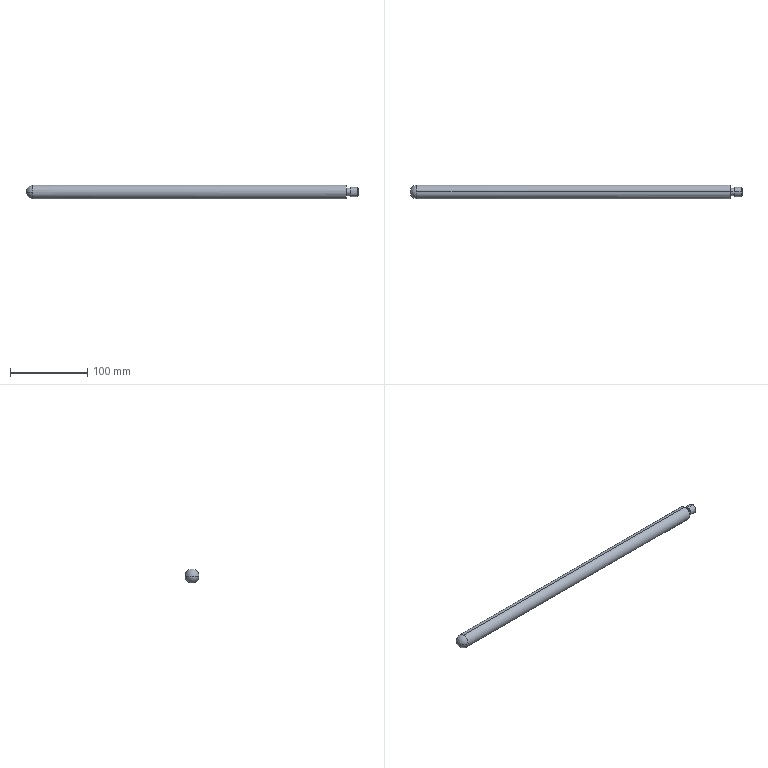Part | SolidWorks | features Chamfer 1, Revolution 1 | 1 solid | 13 faces | box 430 x 18 x 18 mm | volume 106301 mm3 | cylinder 6 | plane 3 | cone 2 | sphere 2 | commonest cylinder face diameters 9.4 x2 12 x2 18 x2
STEP:
#1=CARTESIAN_POINT('',(0.,0.,-5.));
#2=VERTEX_POINT('',#1);
#3=CARTESIAN_POINT('',(0.,0.,5.));
#4=VERTEX_POINT('',#3);
#5=CARTESIAN_POINT('',(0.,0.,0.));
#6=DIRECTION('',(1.,0.,0.));
#7=DIRECTION('',(0.,0.,-1.));
#8=AXIS2_PLACEMENT_3D('',#5,#6,#7);
#9=CIRCLE('',#8,5.);
#10=EDGE_CURVE('',#2,#4,#9,.T.);
#11=ORIENTED_EDGE('',*,*,#10,.F.);
#12=CARTESIAN_POINT('',(-1.,0.,-6.));
#13=VERTEX_POINT('',#12);
#14=CARTESIAN_POINT('',(0.,0.,-5.));
#15=DIRECTION('',(-0.7071,0.,-0.7071));
#16=VECTOR('',#15,1000.);
#17=LINE('',#14,#16);
#18=EDGE_CURVE('',#2,#13,#17,.T.);
#19=ORIENTED_EDGE('',*,*,#18,.T.);
#20=CARTESIAN_POINT('',(-1.,0.,6.));
#21=VERTEX_POINT('',#20);
#22=CARTESIAN_POINT('',(-1.,0.,0.));
#23=DIRECTION('',(-1.,0.,0.));
#24=DIRECTION('',(0.,0.,-1.));
#25=AXIS2_PLACEMENT_3D('',#22,#23,#24);
#26=CIRCLE('',#25,6.);
#27=EDGE_CURVE('',#21,#13,#26,.T.);
#28=ORIENTED_EDGE('',*,*,#27,.F.);
#29=CARTESIAN_POINT('',(0.,0.,5.));
#30=DIRECTION('',(-0.7071,0.,0.7071));
#31=VECTOR('',#30,1000.);
#32=LINE('',#29,#31);
#33=EDGE_CURVE('',#4,#21,#32,.T.);
#34=ORIENTED_EDGE('',*,*,#33,.F.);
#35=EDGE_LOOP('',(#11,#19,#28,#34));
#36=FACE_OUTER_BOUND('',#35,.T.);
#37=CARTESIAN_POINT('',(0.,0.,0.));
#38=DIRECTION('',(-1.,0.,0.));
#39=DIRECTION('',(0.,0.,1.));
#40=AXIS2_PLACEMENT_3D('',#37,#38,#39);
#41=CONICAL_SURFACE('',#40,5.,0.7854);
#42=ADVANCED_FACE('',(#36),#41,.T.);
#43=CARTESIAN_POINT('',(-430.,0.,0.));
#44=VERTEX_POINT('',#43);
#45=CARTESIAN_POINT('',(-421.,9.,0.));
#46=VERTEX_POINT('',#45);
#47=CARTESIAN_POINT('',(-421.,0.,0.));
#48=DIRECTION('',(0.,0.,-1.));
#49=DIRECTION('',(-1.,0.,0.));
#50=AXIS2_PLACEMENT_3D('',#47,#48,#49);
#51=CIRCLE('',#50,9.);
#52=EDGE_CURVE('',#44,#46,#51,.T.);
#53=ORIENTED_EDGE('',*,*,#52,.F.);
#54=CARTESIAN_POINT('',(-421.,-9.,0.));
#55=VERTEX_POINT('',#54);
#56=CARTESIAN_POINT('',(-421.,0.,0.));
#57=DIRECTION('',(0.,0.,1.));
#58=DIRECTION('',(0.,-1.,0.));
#59=AXIS2_PLACEMENT_3D('',#56,#57,#58);
#60=CIRCLE('',#59,9.);
#61=EDGE_CURVE('',#44,#55,#60,.T.);
#62=ORIENTED_EDGE('',*,*,#61,.T.);
#63=CARTESIAN_POINT('',(-421.,0.,9.));
#64=VERTEX_POINT('',#63);
#65=CARTESIAN_POINT('',(-421.,0.,0.));
#66=DIRECTION('',(1.,0.,0.));
#67=DIRECTION('',(0.,0.,-1.));
#68=AXIS2_PLACEMENT_3D('',#65,#66,#67);
#69=CIRCLE('',#68,9.);
#70=EDGE_CURVE('',#64,#55,#69,.T.);
#71=ORIENTED_EDGE('',*,*,#70,.F.);
#72=CARTESIAN_POINT('',(-421.,0.,0.));
#73=DIRECTION('',(1.,0.,0.));
#74=DIRECTION('',(0.,0.,-1.));
#75=AXIS2_PLACEMENT_3D('',#72,#73,#74);
#76=CIRCLE('',#75,9.);
#77=EDGE_CURVE('',#46,#64,#76,.T.);
#78=ORIENTED_EDGE('',*,*,#77,.F.);
#79=EDGE_LOOP('',(#53,#62,#71,#78));
#80=FACE_OUTER_BOUND('',#79,.T.);
#81=CARTESIAN_POINT('',(-421.,0.,0.));
#82=DIRECTION('',(0.,0.,1.));
#83=DIRECTION('',(0.,1.,0.));
#84=AXIS2_PLACEMENT_3D('',#81,#82,#83);
#85=SPHERICAL_SURFACE('',#84,9.);
#86=ADVANCED_FACE('',(#80),#85,.T.);
#87=CARTESIAN_POINT('',(-421.,0.,-9.));
#88=VERTEX_POINT('',#87);
#89=CARTESIAN_POINT('',(-421.,0.,0.));
#90=DIRECTION('',(1.,0.,0.));
#91=DIRECTION('',(0.,0.,-1.));
#92=AXIS2_PLACEMENT_3D('',#89,#90,#91);
#93=CIRCLE('',#92,9.);
#94=EDGE_CURVE('',#88,#46,#93,.T.);
#95=ORIENTED_EDGE('',*,*,#94,.T.);
#96=ORIENTED_EDGE('',*,*,#77,.T.);
#97=CARTESIAN_POINT('',(-15.,0.,9.));
#98=VERTEX_POINT('',#97);
#99=CARTESIAN_POINT('',(-15.,0.,9.));
#100=DIRECTION('',(1.,0.,0.));
#101=VECTOR('',#100,1000.);
#102=LINE('',#99,#101);
#103=EDGE_CURVE('',#64,#98,#102,.T.);
#104=ORIENTED_EDGE('',*,*,#103,.T.);
#105=CARTESIAN_POINT('',(-15.,0.,-9.));
#106=VERTEX_POINT('',#105);
#107=CARTESIAN_POINT('',(-15.,0.,0.));
#108=DIRECTION('',(1.,0.,0.));
#109=DIRECTION('',(0.,0.,-1.));
#110=AXIS2_PLACEMENT_3D('',#107,#108,#109);
#111=CIRCLE('',#110,9.);
#112=EDGE_CURVE('',#106,#98,#111,.T.);
#113=ORIENTED_EDGE('',*,*,#112,.F.);
#114=CARTESIAN_POINT('',(-15.,0.,-9.));
#115=DIRECTION('',(1.,0.,0.));
#116=VECTOR('',#115,1000.);
#117=LINE('',#114,#116);
#118=EDGE_CURVE('',#88,#106,#117,.T.);
#119=ORIENTED_EDGE('',*,*,#118,.F.);
#120=EDGE_LOOP('',(#95,#96,#104,#113,#119));
#121=FACE_OUTER_BOUND('',#120,.T.);
#122=CARTESIAN_POINT('',(-15.,0.,0.));
#123=DIRECTION('',(1.,0.,0.));
#124=DIRECTION('',(0.,0.,-1.));
#125=AXIS2_PLACEMENT_3D('',#122,#123,#124);
#126=CYLINDRICAL_SURFACE('',#125,9.);
#127=ADVANCED_FACE('',(#121),#126,.T.);
#128=CARTESIAN_POINT('',(-15.,0.,-4.7));
#129=VERTEX_POINT('',#128);
#130=CARTESIAN_POINT('',(-15.,0.,4.7));
#131=VERTEX_POINT('',#130);
#132=CARTESIAN_POINT('',(-15.,0.,0.));
#133=DIRECTION('',(1.,0.,0.));
#134=DIRECTION('',(0.,0.,-1.));
#135=AXIS2_PLACEMENT_3D('',#132,#133,#134);
#136=CIRCLE('',#135,4.7);
#137=EDGE_CURVE('',#129,#131,#136,.T.);
#138=ORIENTED_EDGE('',*,*,#137,.T.);
#139=CARTESIAN_POINT('',(-10.,0.,4.7));
#140=VERTEX_POINT('',#139);
#141=CARTESIAN_POINT('',(-15.,0.,4.7));
#142=DIRECTION('',(1.,0.,0.));
#143=VECTOR('',#142,1000.);
#144=LINE('',#141,#143);
#145=EDGE_CURVE('',#131,#140,#144,.T.);
#146=ORIENTED_EDGE('',*,*,#145,.T.);
#147=CARTESIAN_POINT('',(-10.,0.,-4.7));
#148=VERTEX_POINT('',#147);
#149=CARTESIAN_POINT('',(-10.,0.,0.));
#150=DIRECTION('',(1.,0.,0.));
#151=DIRECTION('',(0.,0.,-1.));
#152=AXIS2_PLACEMENT_3D('',#149,#150,#151);
#153=CIRCLE('',#152,4.7);
#154=EDGE_CURVE('',#148,#140,#153,.T.);
#155=ORIENTED_EDGE('',*,*,#154,.F.);
#156=CARTESIAN_POINT('',(-15.,0.,-4.7));
#157=DIRECTION('',(1.,0.,0.));
#158=VECTOR('',#157,1000.);
#159=LINE('',#156,#158);
#160=EDGE_CURVE('',#129,#148,#159,.T.);
#161=ORIENTED_EDGE('',*,*,#160,.F.);
#162=EDGE_LOOP('',(#138,#146,#155,#161));
#163=FACE_OUTER_BOUND('',#162,.T.);
#164=CARTESIAN_POINT('',(-15.,0.,0.));
#165=DIRECTION('',(1.,0.,0.));
#166=DIRECTION('',(0.,0.,-1.));
#167=AXIS2_PLACEMENT_3D('',#164,#165,#166);
#168=CYLINDRICAL_SURFACE('',#167,4.7);
#169=ADVANCED_FACE('',(#163),#168,.T.);
#170=CARTESIAN_POINT('',(-10.,0.,-6.));
#171=VERTEX_POINT('',#170);
#172=CARTESIAN_POINT('',(-10.,0.,6.));
#173=VERTEX_POINT('',#172);
#174=CARTESIAN_POINT('',(-10.,0.,0.));
#175=DIRECTION('',(1.,0.,0.));
#176=DIRECTION('',(0.,0.,-1.));
#177=AXIS2_PLACEMENT_3D('',#174,#175,#176);
#178=CIRCLE('',#177,6.);
#179=EDGE_CURVE('',#171,#173,#178,.T.);
#180=ORIENTED_EDGE('',*,*,#179,.T.);
#181=CARTESIAN_POINT('',(-15.,0.,6.));
#182=DIRECTION('',(1.,0.,0.));
#183=VECTOR('',#182,1000.);
#184=LINE('',#181,#183);
#185=EDGE_CURVE('',#173,#21,#184,.T.);
#186=ORIENTED_EDGE('',*,*,#185,.T.);
#187=ORIENTED_EDGE('',*,*,#27,.T.);
#188=CARTESIAN_POINT('',(-15.,0.,-6.));
#189=DIRECTION('',(1.,0.,0.));
#190=VECTOR('',#189,1000.);
#191=LINE('',#188,#190);
#192=EDGE_CURVE('',#171,#13,#191,.T.);
#193=ORIENTED_EDGE('',*,*,#192,.F.);
#194=EDGE_LOOP('',(#180,#186,#187,#193));
#195=FACE_OUTER_BOUND('',#194,.T.);
#196=CARTESIAN_POINT('',(-15.,0.,0.));
#197=DIRECTION('',(1.,0.,0.));
#198=DIRECTION('',(0.,0.,-1.));
#199=AXIS2_PLACEMENT_3D('',#196,#197,#198);
#200=CYLINDRICAL_SURFACE('',#199,6.);
#201=ADVANCED_FACE('',(#195),#200,.T.);
#202=CARTESIAN_POINT('',(0.,0.,0.));
#203=DIRECTION('',(1.,0.,0.));
#204=DIRECTION('',(0.,0.,-1.));
#205=AXIS2_PLACEMENT_3D('',#202,#203,#204);
#206=CIRCLE('',#205,5.);
#207=EDGE_CURVE('',#4,#2,#206,.T.);
#208=ORIENTED_EDGE('',*,*,#207,.T.);
#209=ORIENTED_EDGE('',*,*,#10,.T.);
#210=EDGE_LOOP('',(#208,#209));
#211=FACE_OUTER_BOUND('',#210,.T.);
#212=CARTESIAN_POINT('',(0.,0.,0.));
#213=DIRECTION('',(1.,0.,0.));
#214=DIRECTION('',(0.,0.,-1.));
#215=AXIS2_PLACEMENT_3D('',#212,#213,#214);
#216=PLANE('',#215);
#217=ADVANCED_FACE('',(#211),#216,.T.);
#218=ORIENTED_EDGE('',*,*,#185,.F.);
#219=CARTESIAN_POINT('',(-10.,0.,0.));
#220=DIRECTION('',(1.,0.,0.));
#221=DIRECTION('',(0.,0.,-1.));
#222=AXIS2_PLACEMENT_3D('',#219,#220,#221);
#223=CIRCLE('',#222,6.);
#224=EDGE_CURVE('',#173,#171,#223,.T.);
#225=ORIENTED_EDGE('',*,*,#224,.T.);
#226=ORIENTED_EDGE('',*,*,#192,.T.);
#227=CARTESIAN_POINT('',(-1.,0.,0.));
#228=DIRECTION('',(-1.,0.,0.));
#229=DIRECTION('',(0.,0.,-1.));
#230=AXIS2_PLACEMENT_3D('',#227,#228,#229);
#231=CIRCLE('',#230,6.);
#232=EDGE_CURVE('',#13,#21,#231,.T.);
#233=ORIENTED_EDGE('',*,*,#232,.T.);
#234=EDGE_LOOP('',(#218,#225,#226,#233));
#235=FACE_OUTER_BOUND('',#234,.T.);
#236=CARTESIAN_POINT('',(-15.,0.,0.));
#237=DIRECTION('',(1.,0.,0.));
#238=DIRECTION('',(0.,0.,-1.));
#239=AXIS2_PLACEMENT_3D('',#236,#237,#238);
#240=CYLINDRICAL_SURFACE('',#239,6.);
#241=ADVANCED_FACE('',(#235),#240,.T.);
#242=ORIENTED_EDGE('',*,*,#154,.T.);
#243=CARTESIAN_POINT('',(-10.,0.,0.));
#244=DIRECTION('',(1.,0.,0.));
#245=DIRECTION('',(0.,0.,-1.));
#246=AXIS2_PLACEMENT_3D('',#243,#244,#245);
#247=CIRCLE('',#246,4.7);
#248=EDGE_CURVE('',#140,#148,#247,.T.);
#249=ORIENTED_EDGE('',*,*,#248,.T.);
#250=EDGE_LOOP('',(#242,#249));
#251=FACE_BOUND('',#250,.T.);
#252=ORIENTED_EDGE('',*,*,#179,.F.);
#253=ORIENTED_EDGE('',*,*,#224,.F.);
#254=EDGE_LOOP('',(#252,#253));
#255=FACE_OUTER_BOUND('',#254,.T.);
#256=CARTESIAN_POINT('',(-10.,4.7,0.));
#257=DIRECTION('',(-1.,0.,0.));
#258=DIRECTION('',(0.,0.,1.));
#259=AXIS2_PLACEMENT_3D('',#256,#257,#258);
#260=PLANE('',#259);
#261=ADVANCED_FACE('',(#251,#255),#260,.T.);
#262=ORIENTED_EDGE('',*,*,#145,.F.);
#263=CARTESIAN_POINT('',(-15.,0.,0.));
#264=DIRECTION('',(1.,0.,0.));
#265=DIRECTION('',(0.,0.,-1.));
#266=AXIS2_PLACEMENT_3D('',#263,#264,#265);
#267=CIRCLE('',#266,4.7);
#268=EDGE_CURVE('',#131,#129,#267,.T.);
#269=ORIENTED_EDGE('',*,*,#268,.T.);
#270=ORIENTED_EDGE('',*,*,#160,.T.);
#271=ORIENTED_EDGE('',*,*,#248,.F.);
#272=EDGE_LOOP('',(#262,#269,#270,#271));
#273=FACE_OUTER_BOUND('',#272,.T.);
#274=CARTESIAN_POINT('',(-15.,0.,0.));
#275=DIRECTION('',(1.,0.,0.));
#276=DIRECTION('',(0.,0.,-1.));
#277=AXIS2_PLACEMENT_3D('',#274,#275,#276);
#278=CYLINDRICAL_SURFACE('',#277,4.7);
#279=ADVANCED_FACE('',(#273),#278,.T.);
#280=ORIENTED_EDGE('',*,*,#112,.T.);
#281=CARTESIAN_POINT('',(-15.,0.,0.));
#282=DIRECTION('',(1.,0.,0.));
#283=DIRECTION('',(0.,0.,-1.));
#284=AXIS2_PLACEMENT_3D('',#281,#282,#283);
#285=CIRCLE('',#284,9.);
#286=EDGE_CURVE('',#98,#106,#285,.T.);
#287=ORIENTED_EDGE('',*,*,#286,.T.);
#288=EDGE_LOOP('',(#280,#287));
#289=FACE_OUTER_BOUND('',#288,.T.);
#290=ORIENTED_EDGE('',*,*,#137,.F.);
#291=ORIENTED_EDGE('',*,*,#268,.F.);
#292=EDGE_LOOP('',(#290,#291));
#293=FACE_BOUND('',#292,.T.);
#294=CARTESIAN_POINT('',(-15.,4.7,0.));
#295=DIRECTION('',(1.,0.,0.));
#296=DIRECTION('',(0.,0.,-1.));
#297=AXIS2_PLACEMENT_3D('',#294,#295,#296);
#298=PLANE('',#297);
#299=ADVANCED_FACE('',(#289,#293),#298,.T.);
#300=ORIENTED_EDGE('',*,*,#103,.F.);
#301=ORIENTED_EDGE('',*,*,#70,.T.);
#302=CARTESIAN_POINT('',(-421.,0.,0.));
#303=DIRECTION('',(1.,0.,0.));
#304=DIRECTION('',(0.,0.,-1.));
#305=AXIS2_PLACEMENT_3D('',#302,#303,#304);
#306=CIRCLE('',#305,9.);
#307=EDGE_CURVE('',#55,#88,#306,.T.);
#308=ORIENTED_EDGE('',*,*,#307,.T.);
#309=ORIENTED_EDGE('',*,*,#118,.T.);
#310=ORIENTED_EDGE('',*,*,#286,.F.);
#311=EDGE_LOOP('',(#300,#301,#308,#309,#310));
#312=FACE_OUTER_BOUND('',#311,.T.);
#313=CARTESIAN_POINT('',(-15.,0.,0.));
#314=DIRECTION('',(1.,0.,0.));
#315=DIRECTION('',(0.,0.,-1.));
#316=AXIS2_PLACEMENT_3D('',#313,#314,#315);
#317=CYLINDRICAL_SURFACE('',#316,9.);
#318=ADVANCED_FACE('',(#312),#317,.T.);
#319=ORIENTED_EDGE('',*,*,#61,.F.);
#320=ORIENTED_EDGE('',*,*,#52,.T.);
#321=ORIENTED_EDGE('',*,*,#94,.F.);
#322=ORIENTED_EDGE('',*,*,#307,.F.);
#323=EDGE_LOOP('',(#319,#320,#321,#322));
#324=FACE_OUTER_BOUND('',#323,.T.);
#325=CARTESIAN_POINT('',(-421.,0.,0.));
#326=DIRECTION('',(0.,0.,1.));
#327=DIRECTION('',(0.,1.,0.));
#328=AXIS2_PLACEMENT_3D('',#325,#326,#327);
#329=SPHERICAL_SURFACE('',#328,9.);
#330=ADVANCED_FACE('',(#324),#329,.T.);
#331=ORIENTED_EDGE('',*,*,#18,.F.);
#332=ORIENTED_EDGE('',*,*,#207,.F.);
#333=ORIENTED_EDGE('',*,*,#33,.T.);
#334=ORIENTED_EDGE('',*,*,#232,.F.);
#335=EDGE_LOOP('',(#331,#332,#333,#334));
#336=FACE_OUTER_BOUND('',#335,.T.);
#337=CARTESIAN_POINT('',(0.,0.,0.));
#338=DIRECTION('',(-1.,0.,0.));
#339=DIRECTION('',(0.,0.,1.));
#340=AXIS2_PLACEMENT_3D('',#337,#338,#339);
#341=CONICAL_SURFACE('',#340,5.,0.7854);
#342=ADVANCED_FACE('',(#336),#341,.T.);
#343=CLOSED_SHELL('',(#42,#86,#127,#169,#201,#217,#241,#261,#279,#299,#318,#330,#342));
#344=MANIFOLD_SOLID_BREP('',#343);
#345=CARTESIAN_POINT('',(0.,0.,0.));
#346=DIRECTION('',(0.,0.,1.));
#347=DIRECTION('',(1.,0.,0.));
#348=AXIS2_PLACEMENT_3D('',#345,#346,#347);
#349=(LENGTH_UNIT()NAMED_UNIT(*)SI_UNIT(.MILLI.,.METRE.));
#350=UNCERTAINTY_MEASURE_WITH_UNIT(LENGTH_MEASURE(0.00001),#349,'','');
#351=(NAMED_UNIT(*)PLANE_ANGLE_UNIT()SI_UNIT($,.RADIAN.));
#352=(NAMED_UNIT(*)SI_UNIT($,.STERADIAN.)SOLID_ANGLE_UNIT());
#353=(GEOMETRIC_REPRESENTATION_CONTEXT(3)GLOBAL_UNCERTAINTY_ASSIGNED_CONTEXT((#350))GLOBAL_UNIT_ASSIGNED_CONTEXT((#349,#351,#352))REPRESENTATION_CONTEXT('',''));
#354=ADVANCED_BREP_SHAPE_REPRESENTATION('',(#344,#348),#353);